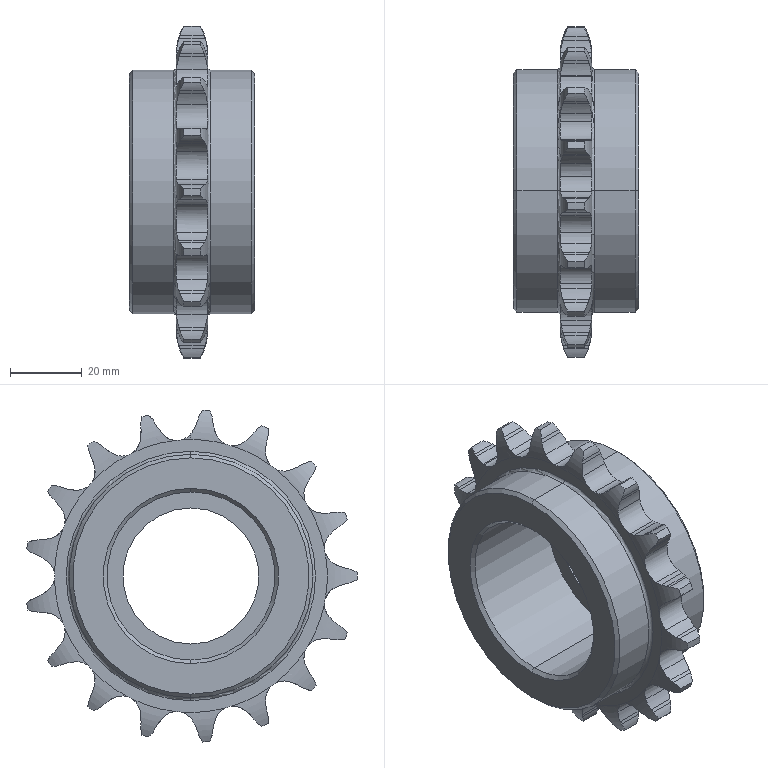Part | NX | features BREP 1 | 1 solid | 205 faces | box 35.002 x 92.378 x 92.763 mm | volume 83391 mm3 | cylinder 118 | torus 40 | plane 39 | cone 8 | commonest cylinder face diameters 14.871 x36 26.567 x35 10.311 x22 93 x17 68 x4 38 x2